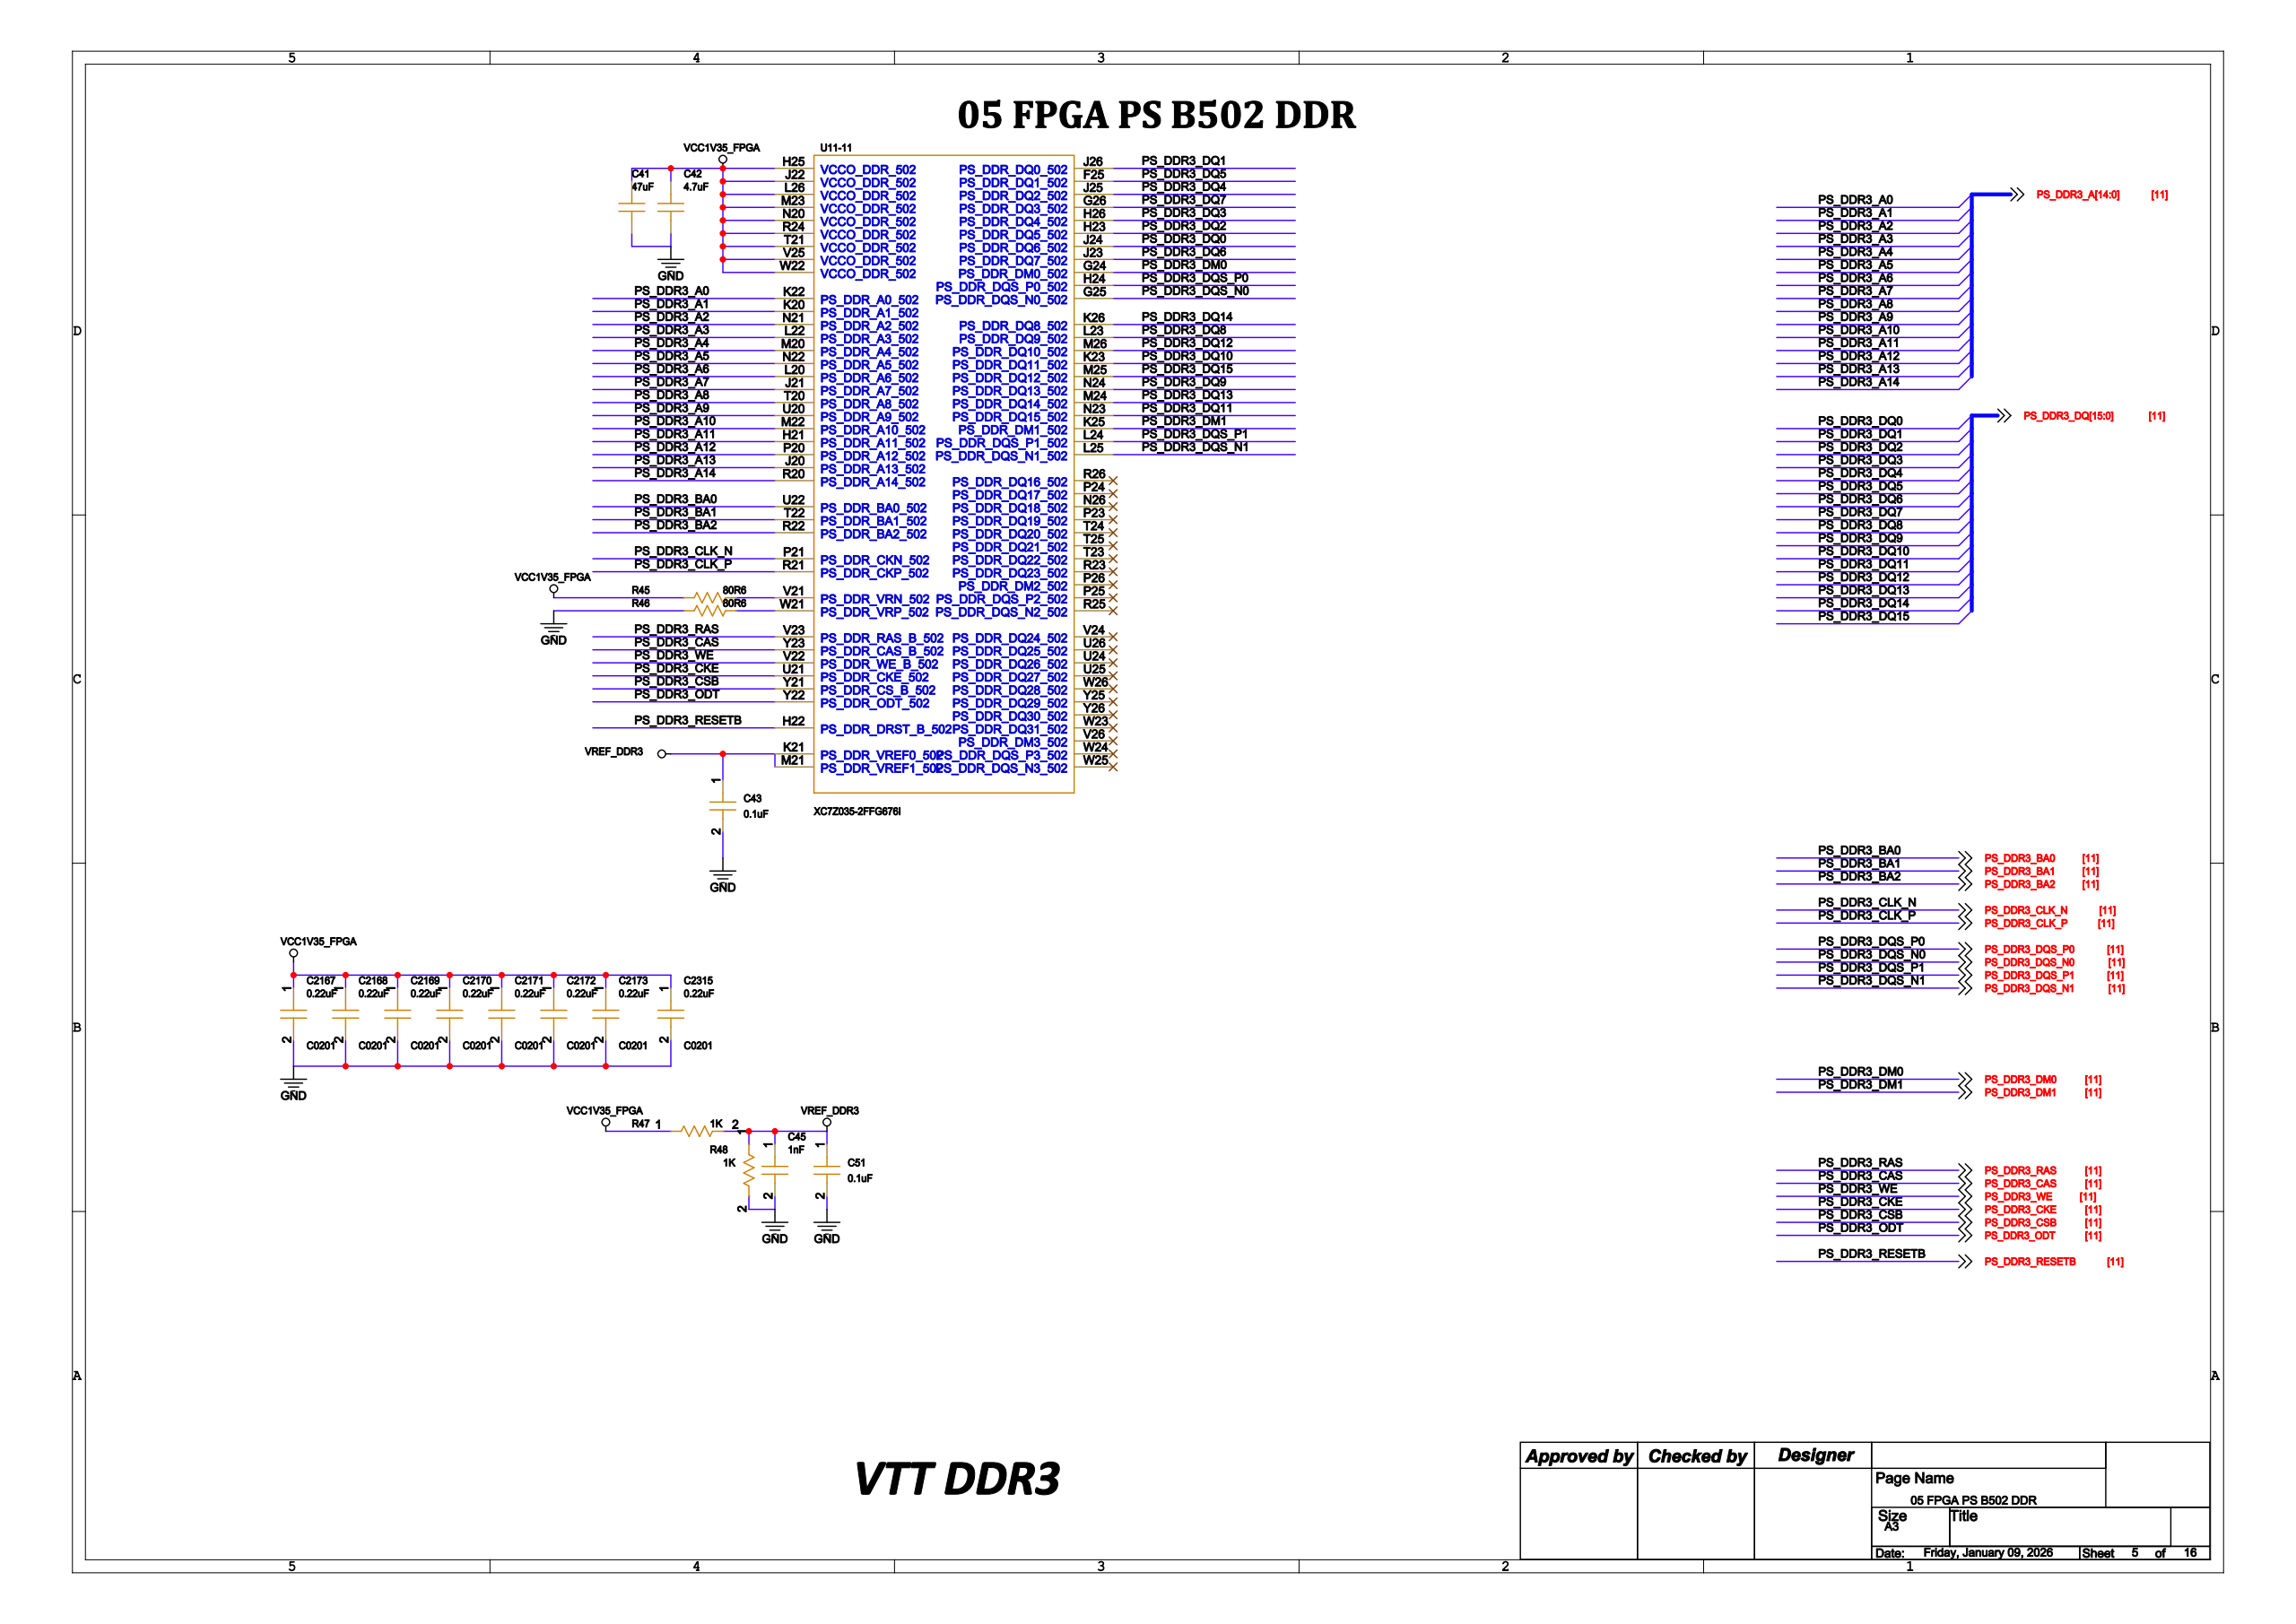Circuit board | Cadence Allegro | 442 parts | 326 nets | one sheet of the schematic
Parts on this sheet (reference | value | footprint):
C41 | 47uF | C0805
C42 | 4.7uF | C0402_D
C43 | 0.1uF | C0201
C45 | 1nF | C0201
C51 | 0.1uF | C0201
C2167 | 0.22uF | C0201
C2168 | 0.22uF | C0201
C2169 | 0.22uF | C0201
C2170 | 0.22uF | C0201
C2171 | 0.22uF | C0201
C2172 | 0.22uF | C0201
C2173 | 0.22uF | C0201
C2315 | 0.22uF | C0201
R45 | 80R6 | R0201
R46 | 80R6 | R0201
R47 | 1K | R0201
R48 | 1K | R0201
Nets of these parts (net: part-pin ...):
GND: C41-2 C42-2 C43-2 C45-2 C51-2 C2167-2 C2168-2 C2169-2 C2170-2 C2171-2 C2172-2 C2173-2 C2315-2 R46-1 R48-2
VCC1V35_FPGA: C41-1 C42-1 C2167-1 C2168-1 C2169-1 C2170-1 C2171-1 C2172-1 C2173-1 C2315-1 R45-1 R47-1
VREF_DDR3: C43-1 C45-1 C51-1 R47-2 R48-1
N50231775: R45-2
N50231777: R46-2